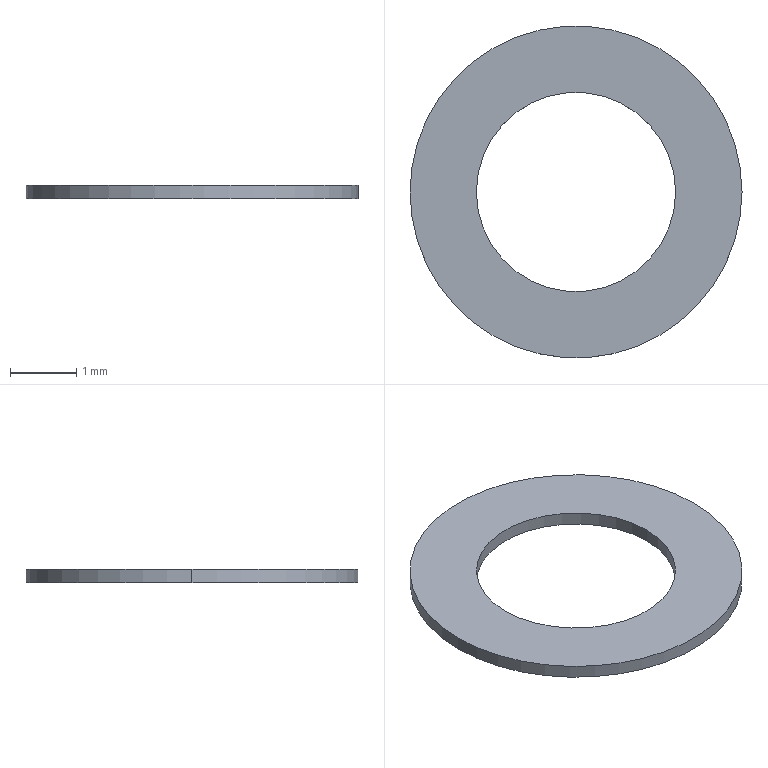Part | SolidWorks | features Extrusion 1 | 1 solid | 6 faces | box 5 x 5 x 0.2 mm | volume 2.513 mm3 | cylinder 4 | plane 2 | commonest cylinder face diameters 3 x2 5 x2
STEP:
#1=CARTESIAN_POINT('',(-1.5,0.,0.2));
#2=VERTEX_POINT('',#1);
#3=CARTESIAN_POINT('',(1.5,0.,0.2));
#4=VERTEX_POINT('',#3);
#5=CARTESIAN_POINT('',(0.,0.,0.2));
#6=DIRECTION('',(0.,0.,1.));
#7=DIRECTION('',(1.,0.,0.));
#8=AXIS2_PLACEMENT_3D('',#5,#6,#7);
#9=CIRCLE('',#8,1.5);
#10=EDGE_CURVE('',#2,#4,#9,.T.);
#11=ORIENTED_EDGE('',*,*,#10,.T.);
#12=CARTESIAN_POINT('',(1.5,0.,0.));
#13=VERTEX_POINT('',#12);
#14=CARTESIAN_POINT('',(1.5,0.,0.2));
#15=DIRECTION('',(0.,0.,-1.));
#16=VECTOR('',#15,1000.);
#17=LINE('',#14,#16);
#18=EDGE_CURVE('',#4,#13,#17,.T.);
#19=ORIENTED_EDGE('',*,*,#18,.T.);
#20=CARTESIAN_POINT('',(-1.5,0.,0.));
#21=VERTEX_POINT('',#20);
#22=CARTESIAN_POINT('',(0.,0.,0.));
#23=DIRECTION('',(0.,0.,1.));
#24=DIRECTION('',(1.,0.,0.));
#25=AXIS2_PLACEMENT_3D('',#22,#23,#24);
#26=CIRCLE('',#25,1.5);
#27=EDGE_CURVE('',#21,#13,#26,.T.);
#28=ORIENTED_EDGE('',*,*,#27,.F.);
#29=CARTESIAN_POINT('',(-1.5,0.,0.2));
#30=DIRECTION('',(0.,0.,-1.));
#31=VECTOR('',#30,1000.);
#32=LINE('',#29,#31);
#33=EDGE_CURVE('',#2,#21,#32,.T.);
#34=ORIENTED_EDGE('',*,*,#33,.F.);
#35=EDGE_LOOP('',(#11,#19,#28,#34));
#36=FACE_OUTER_BOUND('',#35,.T.);
#37=CARTESIAN_POINT('',(0.,0.,0.2));
#38=DIRECTION('',(0.,0.,-1.));
#39=DIRECTION('',(-1.,0.,0.));
#40=AXIS2_PLACEMENT_3D('',#37,#38,#39);
#41=CYLINDRICAL_SURFACE('',#40,1.5);
#42=ADVANCED_FACE('',(#36),#41,.F.);
#43=CARTESIAN_POINT('',(2.5,0.,0.2));
#44=VERTEX_POINT('',#43);
#45=CARTESIAN_POINT('',(-2.5,0.,0.2));
#46=VERTEX_POINT('',#45);
#47=CARTESIAN_POINT('',(0.,0.,0.2));
#48=DIRECTION('',(0.,0.,1.));
#49=DIRECTION('',(1.,0.,0.));
#50=AXIS2_PLACEMENT_3D('',#47,#48,#49);
#51=CIRCLE('',#50,2.5);
#52=EDGE_CURVE('',#44,#46,#51,.T.);
#53=ORIENTED_EDGE('',*,*,#52,.F.);
#54=CARTESIAN_POINT('',(2.5,0.,0.));
#55=VERTEX_POINT('',#54);
#56=CARTESIAN_POINT('',(2.5,0.,0.2));
#57=DIRECTION('',(0.,0.,-1.));
#58=VECTOR('',#57,1000.);
#59=LINE('',#56,#58);
#60=EDGE_CURVE('',#44,#55,#59,.T.);
#61=ORIENTED_EDGE('',*,*,#60,.T.);
#62=CARTESIAN_POINT('',(-2.5,0.,0.));
#63=VERTEX_POINT('',#62);
#64=CARTESIAN_POINT('',(0.,0.,0.));
#65=DIRECTION('',(0.,0.,1.));
#66=DIRECTION('',(1.,0.,0.));
#67=AXIS2_PLACEMENT_3D('',#64,#65,#66);
#68=CIRCLE('',#67,2.5);
#69=EDGE_CURVE('',#55,#63,#68,.T.);
#70=ORIENTED_EDGE('',*,*,#69,.T.);
#71=CARTESIAN_POINT('',(-2.5,0.,0.2));
#72=DIRECTION('',(0.,0.,-1.));
#73=VECTOR('',#72,1000.);
#74=LINE('',#71,#73);
#75=EDGE_CURVE('',#46,#63,#74,.T.);
#76=ORIENTED_EDGE('',*,*,#75,.F.);
#77=EDGE_LOOP('',(#53,#61,#70,#76));
#78=FACE_OUTER_BOUND('',#77,.T.);
#79=CARTESIAN_POINT('',(0.,0.,0.2));
#80=DIRECTION('',(0.,0.,-1.));
#81=DIRECTION('',(-1.,0.,0.));
#82=AXIS2_PLACEMENT_3D('',#79,#80,#81);
#83=CYLINDRICAL_SURFACE('',#82,2.5);
#84=ADVANCED_FACE('',(#78),#83,.T.);
#85=CARTESIAN_POINT('',(0.,0.,0.2));
#86=DIRECTION('',(0.,0.,1.));
#87=DIRECTION('',(1.,0.,0.));
#88=AXIS2_PLACEMENT_3D('',#85,#86,#87);
#89=CIRCLE('',#88,2.5);
#90=EDGE_CURVE('',#46,#44,#89,.T.);
#91=ORIENTED_EDGE('',*,*,#90,.T.);
#92=ORIENTED_EDGE('',*,*,#52,.T.);
#93=EDGE_LOOP('',(#91,#92));
#94=FACE_OUTER_BOUND('',#93,.T.);
#95=ORIENTED_EDGE('',*,*,#10,.F.);
#96=CARTESIAN_POINT('',(0.,0.,0.2));
#97=DIRECTION('',(0.,0.,1.));
#98=DIRECTION('',(1.,0.,0.));
#99=AXIS2_PLACEMENT_3D('',#96,#97,#98);
#100=CIRCLE('',#99,1.5);
#101=EDGE_CURVE('',#4,#2,#100,.T.);
#102=ORIENTED_EDGE('',*,*,#101,.F.);
#103=EDGE_LOOP('',(#95,#102));
#104=FACE_BOUND('',#103,.T.);
#105=CARTESIAN_POINT('',(0.,0.,0.2));
#106=DIRECTION('',(0.,0.,1.));
#107=DIRECTION('',(1.,0.,0.));
#108=AXIS2_PLACEMENT_3D('',#105,#106,#107);
#109=PLANE('',#108);
#110=ADVANCED_FACE('',(#94,#104),#109,.T.);
#111=CARTESIAN_POINT('',(0.,0.,0.));
#112=DIRECTION('',(0.,0.,1.));
#113=DIRECTION('',(1.,0.,0.));
#114=AXIS2_PLACEMENT_3D('',#111,#112,#113);
#115=CIRCLE('',#114,2.5);
#116=EDGE_CURVE('',#63,#55,#115,.T.);
#117=ORIENTED_EDGE('',*,*,#116,.F.);
#118=ORIENTED_EDGE('',*,*,#69,.F.);
#119=EDGE_LOOP('',(#117,#118));
#120=FACE_OUTER_BOUND('',#119,.T.);
#121=ORIENTED_EDGE('',*,*,#27,.T.);
#122=CARTESIAN_POINT('',(0.,0.,0.));
#123=DIRECTION('',(0.,0.,1.));
#124=DIRECTION('',(1.,0.,0.));
#125=AXIS2_PLACEMENT_3D('',#122,#123,#124);
#126=CIRCLE('',#125,1.5);
#127=EDGE_CURVE('',#13,#21,#126,.T.);
#128=ORIENTED_EDGE('',*,*,#127,.T.);
#129=EDGE_LOOP('',(#121,#128));
#130=FACE_BOUND('',#129,.T.);
#131=CARTESIAN_POINT('',(0.,0.,0.));
#132=DIRECTION('',(0.,0.,1.));
#133=DIRECTION('',(1.,0.,0.));
#134=AXIS2_PLACEMENT_3D('',#131,#132,#133);
#135=PLANE('',#134);
#136=ADVANCED_FACE('',(#120,#130),#135,.F.);
#137=ORIENTED_EDGE('',*,*,#60,.F.);
#138=ORIENTED_EDGE('',*,*,#90,.F.);
#139=ORIENTED_EDGE('',*,*,#75,.T.);
#140=ORIENTED_EDGE('',*,*,#116,.T.);
#141=EDGE_LOOP('',(#137,#138,#139,#140));
#142=FACE_OUTER_BOUND('',#141,.T.);
#143=CARTESIAN_POINT('',(0.,0.,0.2));
#144=DIRECTION('',(0.,0.,-1.));
#145=DIRECTION('',(-1.,0.,0.));
#146=AXIS2_PLACEMENT_3D('',#143,#144,#145);
#147=CYLINDRICAL_SURFACE('',#146,2.5);
#148=ADVANCED_FACE('',(#142),#147,.T.);
#149=ORIENTED_EDGE('',*,*,#18,.F.);
#150=ORIENTED_EDGE('',*,*,#101,.T.);
#151=ORIENTED_EDGE('',*,*,#33,.T.);
#152=ORIENTED_EDGE('',*,*,#127,.F.);
#153=EDGE_LOOP('',(#149,#150,#151,#152));
#154=FACE_OUTER_BOUND('',#153,.T.);
#155=CARTESIAN_POINT('',(0.,0.,0.2));
#156=DIRECTION('',(0.,0.,-1.));
#157=DIRECTION('',(-1.,0.,0.));
#158=AXIS2_PLACEMENT_3D('',#155,#156,#157);
#159=CYLINDRICAL_SURFACE('',#158,1.5);
#160=ADVANCED_FACE('',(#154),#159,.F.);
#161=CLOSED_SHELL('',(#42,#84,#110,#136,#148,#160));
#162=MANIFOLD_SOLID_BREP('',#161);
#163=CARTESIAN_POINT('',(0.,0.,0.));
#164=DIRECTION('',(0.,0.,1.));
#165=DIRECTION('',(1.,0.,0.));
#166=AXIS2_PLACEMENT_3D('',#163,#164,#165);
#167=(LENGTH_UNIT()NAMED_UNIT(*)SI_UNIT(.MILLI.,.METRE.));
#168=UNCERTAINTY_MEASURE_WITH_UNIT(LENGTH_MEASURE(0.00001),#167,'','');
#169=(NAMED_UNIT(*)PLANE_ANGLE_UNIT()SI_UNIT($,.RADIAN.));
#170=(NAMED_UNIT(*)SI_UNIT($,.STERADIAN.)SOLID_ANGLE_UNIT());
#171=(GEOMETRIC_REPRESENTATION_CONTEXT(3)GLOBAL_UNCERTAINTY_ASSIGNED_CONTEXT((#168))GLOBAL_UNIT_ASSIGNED_CONTEXT((#167,#169,#170))REPRESENTATION_CONTEXT('',''));
#172=ADVANCED_BREP_SHAPE_REPRESENTATION('',(#162,#166),#171);